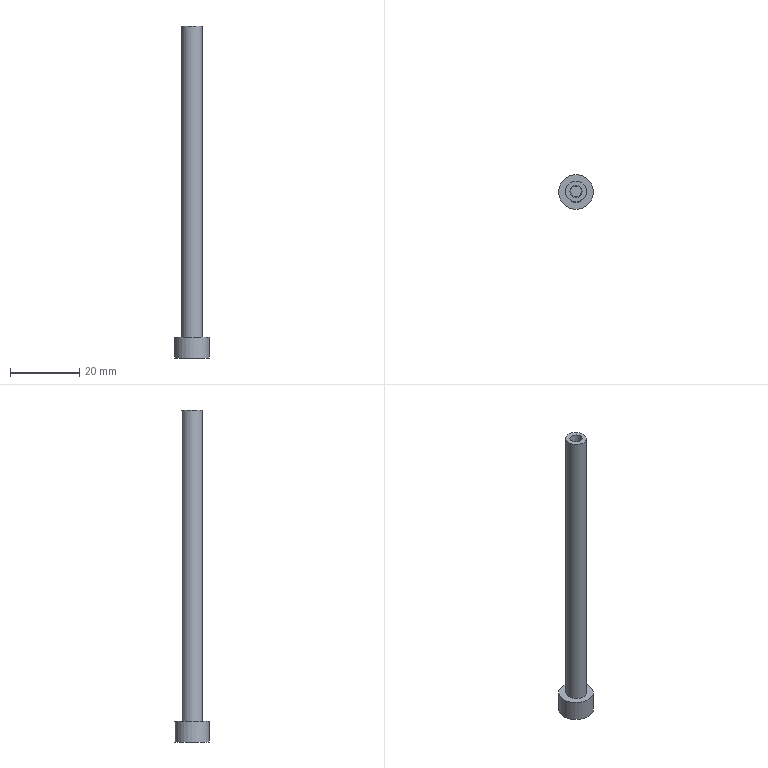Part | NX | features solid 2 | 1 solid | 7 faces | box 10 x 10 x 95.81 mm | volume 2980 mm3 | plane 4 | cylinder 2 | cone 1 | commonest cylinder face diameters 6 x1 10 x1
STEP:
#1=CARTESIAN_POINT('',(-27.15,0.,25.81));
#2=VERTEX_POINT('',#1);
#3=CARTESIAN_POINT('',(-30.15,0.,25.81));
#4=DIRECTION('',(0.,0.,1.));
#5=DIRECTION('',(1.,0.,0.));
#6=AXIS2_PLACEMENT_3D('',#3,#4,#5);
#7=CIRCLE('',#6,3.);
#8=EDGE_CURVE('',#2,#2,#7,.F.);
#9=ORIENTED_EDGE('',*,*,#8,.F.);
#10=EDGE_LOOP('',(#9));
#11=FACE_BOUND('',#10,.T.);
#12=CARTESIAN_POINT('',(-28.4,0.,25.81));
#13=VERTEX_POINT('',#12);
#14=CARTESIAN_POINT('',(-30.15,0.,25.81));
#15=DIRECTION('',(0.,0.,1.));
#16=DIRECTION('',(1.,0.,0.));
#17=AXIS2_PLACEMENT_3D('',#14,#15,#16);
#18=CIRCLE('',#17,1.75);
#19=EDGE_CURVE('',#13,#13,#18,.F.);
#20=ORIENTED_EDGE('',*,*,#19,.T.);
#21=EDGE_LOOP('',(#20));
#22=FACE_BOUND('',#21,.T.);
#23=CARTESIAN_POINT('',(0.,0.,25.81));
#24=DIRECTION('',(0.,0.,1.));
#25=DIRECTION('',(0.,-1.,0.));
#26=AXIS2_PLACEMENT_3D('',#23,#24,#25);
#27=PLANE('',#26);
#28=ADVANCED_FACE('',(#11,#22),#27,.T.);
#29=CARTESIAN_POINT('',(-25.15,0.,-70.));
#30=VERTEX_POINT('',#29);
#31=CARTESIAN_POINT('',(-30.15,0.,-70.));
#32=DIRECTION('',(0.,0.,1.));
#33=DIRECTION('',(1.,0.,0.));
#34=AXIS2_PLACEMENT_3D('',#31,#32,#33);
#35=CIRCLE('',#34,5.);
#36=EDGE_CURVE('',#30,#30,#35,.T.);
#37=ORIENTED_EDGE('',*,*,#36,.F.);
#38=EDGE_LOOP('',(#37));
#39=FACE_BOUND('',#38,.T.);
#40=CARTESIAN_POINT('',(0.,0.,-70.));
#41=DIRECTION('',(0.,0.,-1.));
#42=DIRECTION('',(-1.,0.,0.));
#43=AXIS2_PLACEMENT_3D('',#40,#41,#42);
#44=PLANE('',#43);
#45=ADVANCED_FACE('',(#39),#44,.T.);
#46=CARTESIAN_POINT('',(-25.15,0.,-64.));
#47=VERTEX_POINT('',#46);
#48=CARTESIAN_POINT('',(-30.15,0.,-64.));
#49=DIRECTION('',(0.,0.,1.));
#50=DIRECTION('',(1.,0.,0.));
#51=AXIS2_PLACEMENT_3D('',#48,#49,#50);
#52=CIRCLE('',#51,5.);
#53=EDGE_CURVE('',#47,#47,#52,.T.);
#54=ORIENTED_EDGE('',*,*,#53,.F.);
#55=EDGE_LOOP('',(#54));
#56=FACE_BOUND('',#55,.T.);
#57=ORIENTED_EDGE('',*,*,#36,.T.);
#58=EDGE_LOOP('',(#57));
#59=FACE_BOUND('',#58,.T.);
#60=CARTESIAN_POINT('',(-30.15,0.,-64.));
#61=DIRECTION('',(0.,0.,-1.));
#62=DIRECTION('',(-1.,0.,0.));
#63=AXIS2_PLACEMENT_3D('',#60,#61,#62);
#64=CYLINDRICAL_SURFACE('',#63,5.);
#65=ADVANCED_FACE('',(#56,#59),#64,.T.);
#66=CARTESIAN_POINT('',(-27.15,0.,-64.));
#67=VERTEX_POINT('',#66);
#68=CARTESIAN_POINT('',(-30.15,0.,-64.));
#69=DIRECTION('',(0.,0.,1.));
#70=DIRECTION('',(1.,0.,0.));
#71=AXIS2_PLACEMENT_3D('',#68,#69,#70);
#72=CIRCLE('',#71,3.);
#73=EDGE_CURVE('',#67,#67,#72,.F.);
#74=ORIENTED_EDGE('',*,*,#73,.T.);
#75=EDGE_LOOP('',(#74));
#76=FACE_BOUND('',#75,.T.);
#77=ORIENTED_EDGE('',*,*,#53,.T.);
#78=EDGE_LOOP('',(#77));
#79=FACE_BOUND('',#78,.T.);
#80=CARTESIAN_POINT('',(-30.15,0.,-64.));
#81=DIRECTION('',(0.,0.,1.));
#82=DIRECTION('',(1.,0.,0.));
#83=AXIS2_PLACEMENT_3D('',#80,#81,#82);
#84=PLANE('',#83);
#85=ADVANCED_FACE('',(#76,#79),#84,.T.);
#86=ORIENTED_EDGE('',*,*,#8,.T.);
#87=EDGE_LOOP('',(#86));
#88=FACE_BOUND('',#87,.T.);
#89=ORIENTED_EDGE('',*,*,#73,.F.);
#90=EDGE_LOOP('',(#89));
#91=FACE_BOUND('',#90,.T.);
#92=CARTESIAN_POINT('',(-30.15,0.,40.81));
#93=DIRECTION('',(0.,0.,-1.));
#94=DIRECTION('',(-1.,0.,0.));
#95=AXIS2_PLACEMENT_3D('',#92,#93,#94);
#96=CYLINDRICAL_SURFACE('',#95,3.);
#97=ADVANCED_FACE('',(#88,#91),#96,.T.);
#98=CARTESIAN_POINT('',(-31.717,0.,22.31));
#99=VERTEX_POINT('',#98);
#100=CARTESIAN_POINT('',(-30.15,0.,22.31));
#101=DIRECTION('',(0.,0.,-1.));
#102=DIRECTION('',(-1.,0.,0.));
#103=AXIS2_PLACEMENT_3D('',#100,#101,#102);
#104=CIRCLE('',#103,1.567);
#105=EDGE_CURVE('',#99,#99,#104,.F.);
#106=ORIENTED_EDGE('',*,*,#105,.F.);
#107=EDGE_LOOP('',(#106));
#108=FACE_BOUND('',#107,.T.);
#109=ORIENTED_EDGE('',*,*,#19,.F.);
#110=EDGE_LOOP('',(#109));
#111=FACE_BOUND('',#110,.T.);
#112=CARTESIAN_POINT('',(-30.15,0.,25.81));
#113=DIRECTION('',(0.,0.,1.));
#114=DIRECTION('',(1.,0.,0.));
#115=AXIS2_PLACEMENT_3D('',#112,#113,#114);
#116=CONICAL_SURFACE('',#115,1.75,0.05236);
#117=ADVANCED_FACE('',(#108,#111),#116,.F.);
#118=ORIENTED_EDGE('',*,*,#105,.T.);
#119=EDGE_LOOP('',(#118));
#120=FACE_BOUND('',#119,.T.);
#121=CARTESIAN_POINT('',(-30.15,0.,22.31));
#122=DIRECTION('',(0.,0.,-1.));
#123=DIRECTION('',(-1.,0.,0.));
#124=AXIS2_PLACEMENT_3D('',#121,#122,#123);
#125=PLANE('',#124);
#126=ADVANCED_FACE('',(#120),#125,.F.);
#127=CLOSED_SHELL('',(#28,#45,#65,#85,#97,#117,#126));
#128=MANIFOLD_SOLID_BREP('',#127);
#129=(LENGTH_UNIT()NAMED_UNIT(*)SI_UNIT(.MILLI.,.METRE.));
#130=UNCERTAINTY_MEASURE_WITH_UNIT(LENGTH_MEASURE(0.00001),#129,'','');
#131=(NAMED_UNIT(*)PLANE_ANGLE_UNIT()SI_UNIT($,.RADIAN.));
#132=(NAMED_UNIT(*)SI_UNIT($,.STERADIAN.)SOLID_ANGLE_UNIT());
#133=(GEOMETRIC_REPRESENTATION_CONTEXT(3)GLOBAL_UNCERTAINTY_ASSIGNED_CONTEXT((#130))GLOBAL_UNIT_ASSIGNED_CONTEXT((#129,#131,#132))REPRESENTATION_CONTEXT('',''));
#134=ADVANCED_BREP_SHAPE_REPRESENTATION('',(#128),#133);